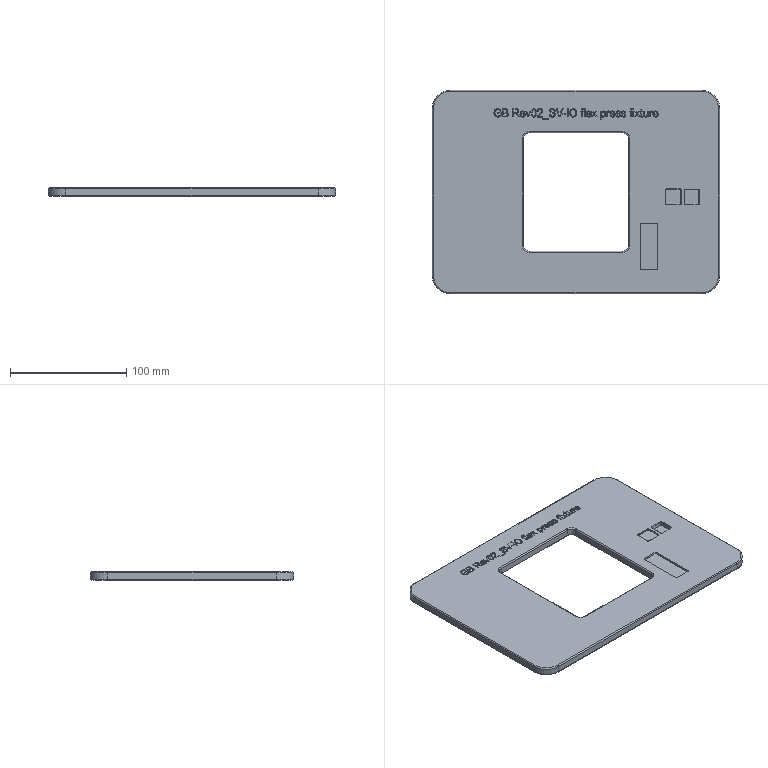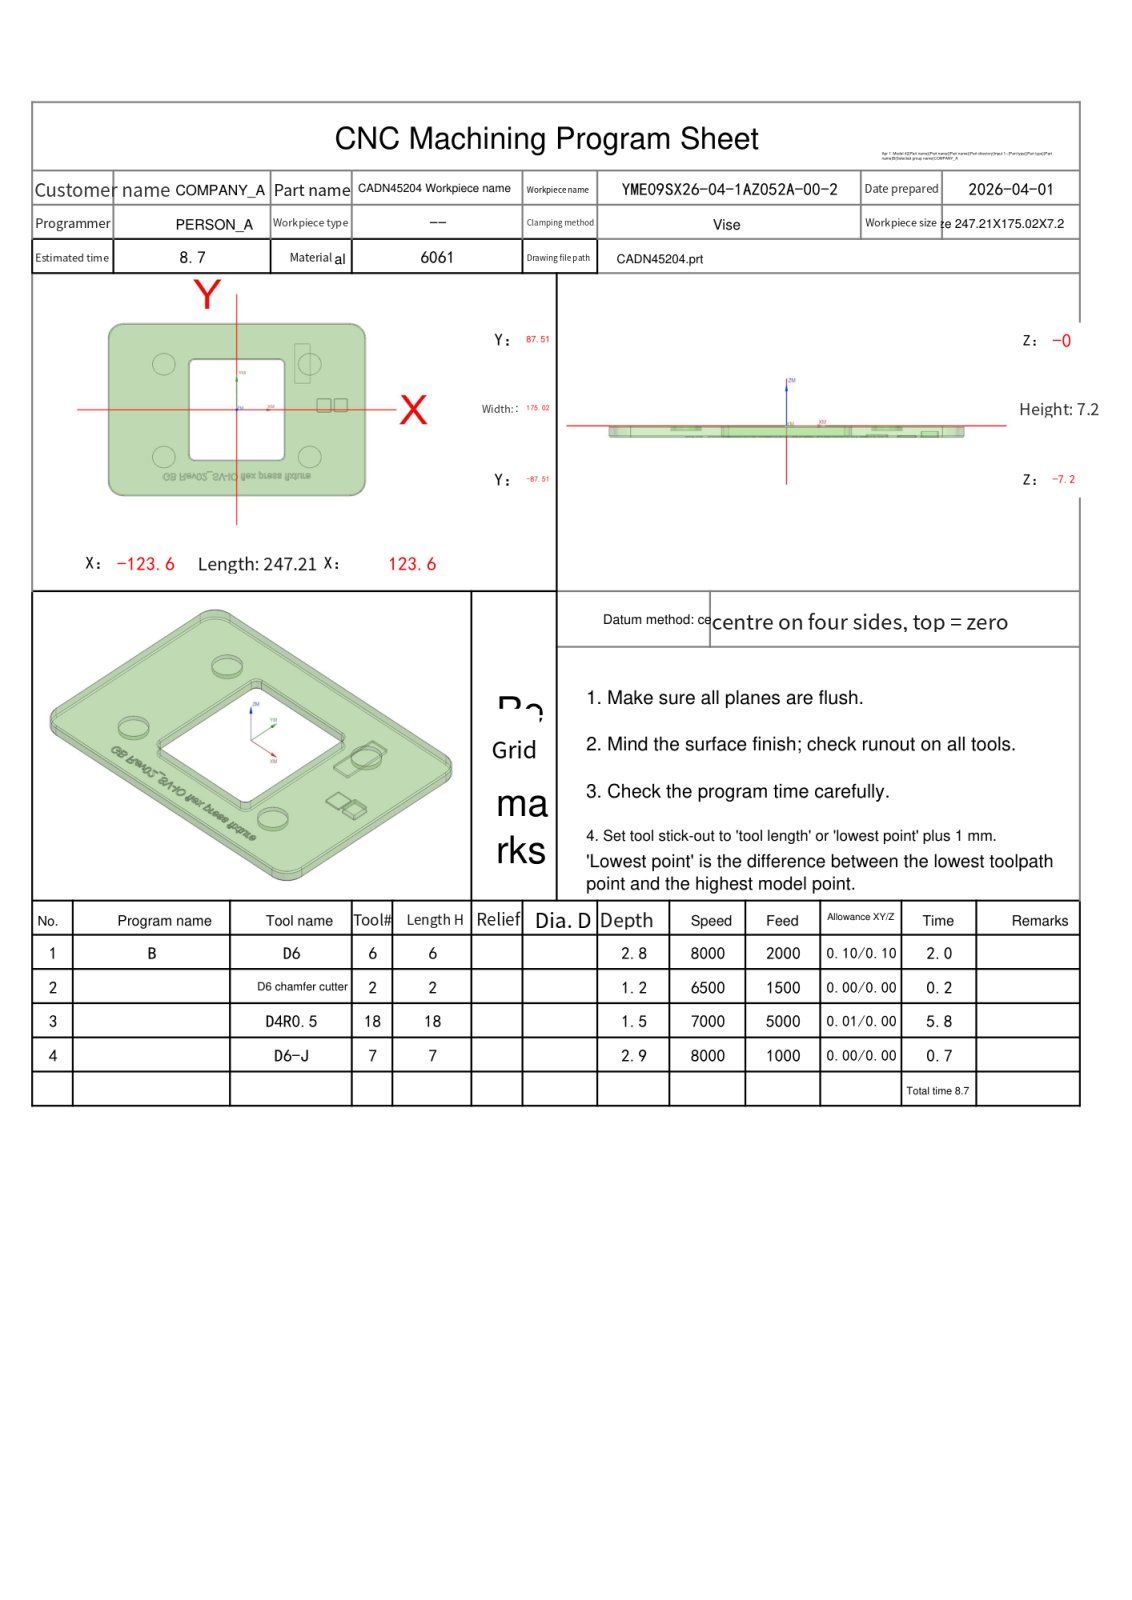NC program | NX | posted by the shop | part box 247.208 x 175.016 x 7.2 mm
Lines 22683 to 22917 of 22917:
N4 T07 M06
(D6-J  D=6. R=0. H=07 ce=0.40 di=0.00)
G00 G90 G54 X74.6 Y-47.743 M03 S8000
G43 H07 Z10.4
M08
Z-.9
G01 Y-48.279 Z-1.044 F1000.
X74.471 Y-49.097 Z-1.265
X74.199 Y-49.879 Z-1.487
X73.79 Y-50.599 Z-1.709
X73.26 Y-51.235 Z-1.931
X72.624 Y-51.766 Z-2.153
X71.903 Y-52.174 Z-2.375
X71.122 Y-52.447 Z-2.597
X70.303 Y-52.575 Z-2.819
X70. Z-2.9
Y-55.575
G02 X62.4 Y-47.975 I0.0 J7.6
X70. Y-40.375 I7.6 J0.0
X77.6 Y-47.975 I0.0 J-7.6
X70. Y-55.575 I-7.6 J0.0
X67.464 Y-55.14 I0.0 J7.6
X67.065 Y-54.593 I.2 J.566
G01 X66.972 Y-51.682
G03 X66.791 Y-51.271 I-.6 J-.019
G02 X65.4 Y-47.975 I3.209 J3.296
X70. Y-43.375 I4.6 J0.0
X74.6 Y-47.975 I0.0 J-4.6
X70.264 Y-52.568 I-4.6 J0.0
G01 X70.23 Y-52.569
G02 X69.633 Y-52.026 I0.0 J.6
G01 X69.416 Y-49.773
G03 X69.141 Y-49.325 I-.597 J-.058
G02 X68.4 Y-47.975 I.859 J1.35
X70. Y-46.375 I1.6 J0.0
X71.6 Y-47.975 I0.0 J-1.6
X70. Y-49.575 I-1.6 J0.0
X69.385 Y-49.452 I0.0 J1.6
X68.637 Y-48.813 I.615 J1.477
G03 X67.614 Y-48.241 I-1.022 J-.628
X66.986 Y-48.419 I0.0 J-1.2
G01 Z-1.4
G00 Z10.4
X65.4 Y45.793
Z-.9
G01 Y46.328 Z-1.044
X65.529 Y47.146 Z-1.265
X65.801 Y47.928 Z-1.487
X66.21 Y48.649 Z-1.709
X66.74 Y49.284 Z-1.931
X67.376 Y49.815 Z-2.153
X68.097 Y50.223 Z-2.375
X68.878 Y50.496 Z-2.597
X69.697 Y50.625 Z-2.819
X70. Z-2.9
Y53.625
G02 X77.6 Y46.025 I0.0 J-7.6
X70. Y38.425 I-7.6 J0.0
X62.4 Y46.025 I0.0 J7.6
X70. Y53.625 I7.6 J0.0
X72.536 Y53.189 I0.0 J-7.6
X72.935 Y52.643 I-.2 J-.566
G01 X73.028 Y49.731
G03 X73.209 Y49.32 I.6 J.019
G02 X74.6 Y46.025 I-3.209 J-3.296
X70. Y41.425 I-4.6 J0.0
X65.4 Y46.025 I0.0 J4.6
X69.736 Y50.617 I4.6 J0.0
G01 X69.77 Y50.618
G02 X70.367 Y50.076 I0.0 J-.6
G01 X70.584 Y47.823
G03 X70.859 Y47.374 I.597 J.058
G02 X71.6 Y46.025 I-.859 J-1.35
X70. Y44.425 I-1.6 J0.0
X68.4 Y46.025 I0.0 J1.6
X70. Y47.625 I1.6 J0.0
X70.615 Y47.502 I0.0 J-1.6
X71.363 Y46.862 I-.615 J-1.477
G03 X72.386 Y46.291 I1.022 J.628
X73.014 Y46.468 I0.0 J1.2
G01 Z-1.4
G00 Z10.4
X-74.6 Y45.793
Z-.9
G01 Y46.328 Z-1.044
X-74.471 Y47.146 Z-1.265
X-74.199 Y47.928 Z-1.487
X-73.79 Y48.649 Z-1.709
X-73.26 Y49.284 Z-1.931
X-72.624 Y49.815 Z-2.153
X-71.903 Y50.223 Z-2.375
X-71.122 Y50.496 Z-2.597
X-70.303 Y50.625 Z-2.819
X-70. Z-2.9
Y53.625
G02 X-62.4 Y46.025 I0.0 J-7.6
X-70. Y38.425 I-7.6 J0.0
X-77.6 Y46.025 I0.0 J7.6
X-70. Y53.625 I7.6 J0.0
X-67.464 Y53.189 I0.0 J-7.6
X-67.065 Y52.643 I-.2 J-.566
G01 X-66.972 Y49.731
G03 X-66.791 Y49.32 I.6 J.019
G02 X-65.4 Y46.025 I-3.209 J-3.296
X-70. Y41.425 I-4.6 J0.0
X-74.6 Y46.025 I0.0 J4.6
X-70.264 Y50.617 I4.6 J0.0
G01 X-70.23 Y50.618
G02 X-69.633 Y50.076 I0.0 J-.6
G01 X-69.416 Y47.823
G03 X-69.141 Y47.374 I.597 J.058
G02 X-68.4 Y46.025 I-.859 J-1.35
X-70. Y44.425 I-1.6 J0.0
X-71.6 Y46.025 I0.0 J1.6
X-70. Y47.625 I1.6 J0.0
X-69.385 Y47.502 I0.0 J-1.6
X-68.637 Y46.862 I-.615 J-1.477
G03 X-67.614 Y46.291 I1.022 J.628
X-66.986 Y46.468 I0.0 J1.2
G01 Z-1.4
G00 Z10.4
X-65.4 Y-47.743
Z-.9
G01 Y-48.279 Z-1.044
X-65.529 Y-49.097 Z-1.265
X-65.801 Y-49.879 Z-1.487
X-66.21 Y-50.599 Z-1.709
X-66.74 Y-51.235 Z-1.931
X-67.376 Y-51.766 Z-2.153
X-68.097 Y-52.174 Z-2.375
X-68.878 Y-52.447 Z-2.597
X-69.697 Y-52.575 Z-2.819
X-70. Z-2.9
Y-55.575
G02 X-77.6 Y-47.975 I0.0 J7.6
X-70. Y-40.375 I7.6 J0.0
X-62.4 Y-47.975 I0.0 J-7.6
X-70. Y-55.575 I-7.6 J0.0
X-72.536 Y-55.14 I0.0 J7.6
X-72.935 Y-54.593 I.2 J.566
G01 X-73.028 Y-51.682
G03 X-73.209 Y-51.271 I-.6 J-.019
G02 X-74.6 Y-47.975 I3.209 J3.296
X-70. Y-43.375 I4.6 J0.0
X-65.4 Y-47.975 I0.0 J-4.6
X-69.736 Y-52.568 I-4.6 J0.0
G01 X-69.77 Y-52.569
G02 X-70.367 Y-52.026 I0.0 J.6
G01 X-70.584 Y-49.773
G03 X-70.859 Y-49.325 I-.597 J-.058
G02 X-71.6 Y-47.975 I.859 J1.35
X-70. Y-46.375 I1.6 J0.0
X-68.4 Y-47.975 I0.0 J-1.6
X-70. Y-49.575 I-1.6 J0.0
X-70.615 Y-49.452 I0.0 J1.6
X-71.363 Y-48.813 I.615 J1.477
G03 X-72.386 Y-48.241 I-1.022 J-.628
X-73.014 Y-48.419 I0.0 J-1.2
G01 Z-1.4
G00 Z10.4
G00 G90 X68.8 Y-54.469 M03 S8000
Z10.
Z-1.9
G01 Z-2.9 F1000.
G41 D07
Y-54.775
G03 X70. Y-55.975 I1.2 J0.0
X78. Y-47.975 I0.0 J8.
X70. Y-39.975 I-8. J0.0
X62. Y-47.975 I0.0 J-8.
X70. Y-55.975 I8. J0.0
X70.4 Y-55.965 I0.0 J8.
X71.54 Y-54.767 I-.06 J1.199
G01 X71.538 Y-54.707
X71.533 Y-54.6
G40 X71.523 Y-54.401
Z-1.9
G00 Z10.
X71.2 Y52.518
Z-1.9
G01 Z-2.9
G41 D07
Y52.825
G03 X70. Y54.025 I-1.2 J0.0
X62. Y46.025 I0.0 J-8.
X70. Y38.025 I8. J0.0
X78. Y46.025 I0.0 J8.
X70. Y54.025 I-8. J0.0
X69.6 Y54.015 I0.0 J-8.
X68.46 Y52.816 I.06 J-1.199
G01 X68.462 Y52.756
X68.467 Y52.65
G40 X68.477 Y52.45
Z-1.9
G00 Z10.
X-68.8 Y52.518
Z-1.9
G01 Z-2.9
G41 D07
Y52.825
G03 X-70. Y54.025 I-1.2 J0.0
X-78. Y46.025 I0.0 J-8.
X-70. Y38.025 I8. J0.0
X-62. Y46.025 I0.0 J8.
X-70. Y54.025 I-8. J0.0
X-70.4 Y54.015 I0.0 J-8.
X-71.54 Y52.816 I.06 J-1.199
G01 X-71.538 Y52.756
X-71.533 Y52.65
G40 X-71.523 Y52.45
Z-1.9
G00 Z10.
X-71.2 Y-54.469
Z-1.9
G01 Z-2.9
G41 D07
Y-54.775
G03 X-70. Y-55.975 I1.2 J0.0
X-62. Y-47.975 I0.0 J8.
X-70. Y-39.975 I-8. J0.0
X-78. Y-47.975 I0.0 J-8.
X-70. Y-55.975 I8. J0.0
X-69.6 Y-55.965 I0.0 J8.
X-68.46 Y-54.767 I-.06 J1.199
G01 X-68.462 Y-54.707
X-68.467 Y-54.6
G40 X-68.477 Y-54.401
Z-1.9
G00 Z10.
M05
M09
G91 G28 Z0.0
G91 G28 Y0.0
M30
%